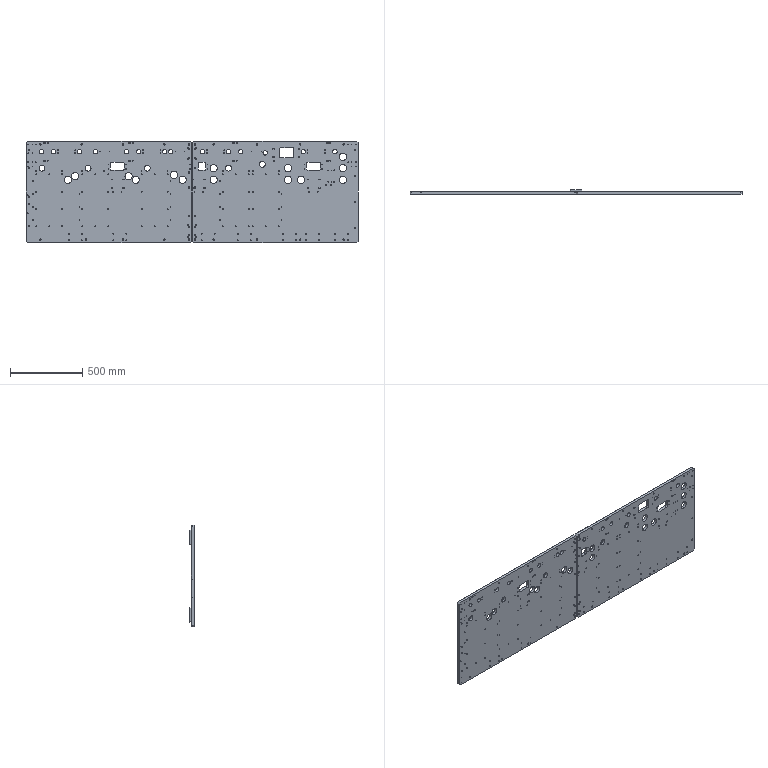Part | NX | 4 solids | 1434 faces | box 2300 x 32 x 700 mm | volume 30828054 mm3 | cylinder 764 | cone 548 | plane 122 | commonest cylinder face diameters 6.8 x184 5 x112 4.2 x96 16 x82 10 x68 3.3 x44